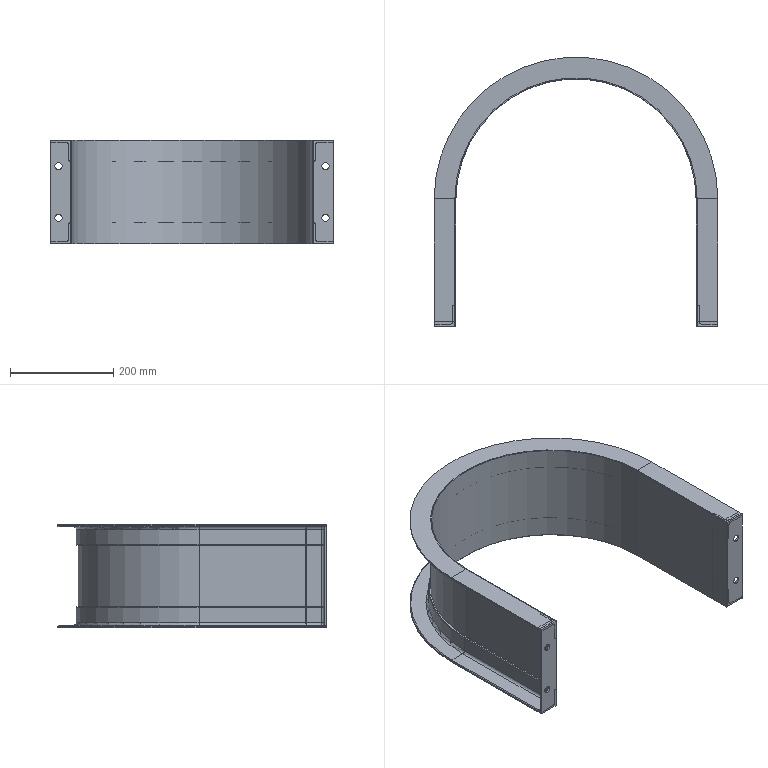Part | STEP file | Coupling guard_Default<As machined> | 13 solids | 150 faces | box 550 x 522 x 200 mm | volume 1395194 mm3 | plane 98 | cylinder 46 | torus 6 | commonest cylinder face diameters 2.667 x16 10 x10 14 x8 2.64 x4 470 x3 478 x2